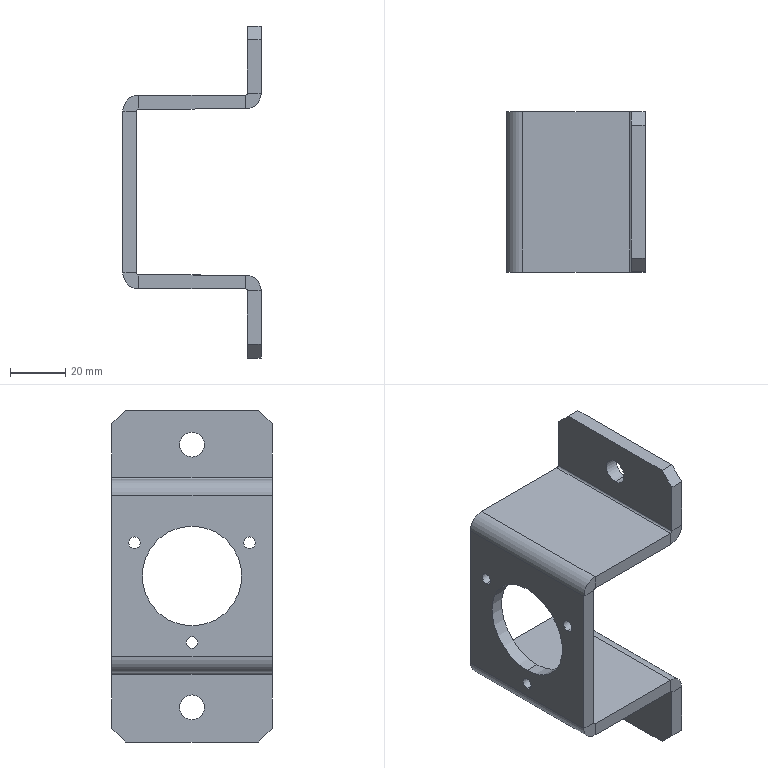Part | SolidWorks | features EdgeFlange 2, HoleWzd 2, Chamfer 1, CirPattern 1, FlatPattern 1, ICE 1, SMBaseFlange 1, SheetMetal 1 | 1 solid | 54 faces | box 50 x 58 x 120 mm | volume 53105 mm3 | plane 34 | cylinder 20 | commonest cylinder face diameters 4.2 x6 1.473 x4 9 x4 11.473 x4 36 x2
STEP:
#1=CARTESIAN_POINT('',(0.,20.785,14.1));
#2=VERTEX_POINT('',#1);
#3=CARTESIAN_POINT('',(0.,20.785,9.9));
#4=VERTEX_POINT('',#3);
#5=CARTESIAN_POINT('',(0.,20.785,12.));
#6=DIRECTION('',(1.,0.,0.));
#7=DIRECTION('',(0.,0.,-1.));
#8=AXIS2_PLACEMENT_3D('',#5,#6,#7);
#9=CIRCLE('',#8,2.1);
#10=EDGE_CURVE('',#2,#4,#9,.T.);
#11=ORIENTED_EDGE('',*,*,#10,.T.);
#12=CARTESIAN_POINT('',(-5.,20.785,9.9));
#13=VERTEX_POINT('',#12);
#14=CARTESIAN_POINT('',(-5.,20.785,9.9));
#15=DIRECTION('',(-1.,0.,0.));
#16=VECTOR('',#15,1000.);
#17=LINE('',#14,#16);
#18=EDGE_CURVE('',#4,#13,#17,.T.);
#19=ORIENTED_EDGE('',*,*,#18,.T.);
#20=CARTESIAN_POINT('',(-5.,20.785,14.1));
#21=VERTEX_POINT('',#20);
#22=CARTESIAN_POINT('',(-5.,20.785,12.));
#23=DIRECTION('',(-1.,0.,0.));
#24=DIRECTION('',(0.,0.,1.));
#25=AXIS2_PLACEMENT_3D('',#22,#23,#24);
#26=CIRCLE('',#25,2.1);
#27=EDGE_CURVE('',#13,#21,#26,.T.);
#28=ORIENTED_EDGE('',*,*,#27,.T.);
#29=CARTESIAN_POINT('',(-5.,20.785,14.1));
#30=DIRECTION('',(-1.,0.,0.));
#31=VECTOR('',#30,1000.);
#32=LINE('',#29,#31);
#33=EDGE_CURVE('',#2,#21,#32,.T.);
#34=ORIENTED_EDGE('',*,*,#33,.F.);
#35=EDGE_LOOP('',(#11,#19,#28,#34));
#36=FACE_OUTER_BOUND('',#35,.T.);
#37=CARTESIAN_POINT('',(-5.,20.785,12.));
#38=DIRECTION('',(-1.,0.,0.));
#39=DIRECTION('',(0.,0.,1.));
#40=AXIS2_PLACEMENT_3D('',#37,#38,#39);
#41=CYLINDRICAL_SURFACE('',#40,2.1);
#42=ADVANCED_FACE('',(#36),#41,.F.);
#43=CARTESIAN_POINT('',(0.,-20.785,14.1));
#44=VERTEX_POINT('',#43);
#45=CARTESIAN_POINT('',(0.,-20.785,9.9));
#46=VERTEX_POINT('',#45);
#47=CARTESIAN_POINT('',(0.,-20.785,12.));
#48=DIRECTION('',(1.,0.,0.));
#49=DIRECTION('',(0.,0.,-1.));
#50=AXIS2_PLACEMENT_3D('',#47,#48,#49);
#51=CIRCLE('',#50,2.1);
#52=EDGE_CURVE('',#44,#46,#51,.T.);
#53=ORIENTED_EDGE('',*,*,#52,.T.);
#54=CARTESIAN_POINT('',(-5.,-20.785,9.9));
#55=VERTEX_POINT('',#54);
#56=CARTESIAN_POINT('',(-5.,-20.785,9.9));
#57=DIRECTION('',(-1.,0.,0.));
#58=VECTOR('',#57,1000.);
#59=LINE('',#56,#58);
#60=EDGE_CURVE('',#46,#55,#59,.T.);
#61=ORIENTED_EDGE('',*,*,#60,.T.);
#62=CARTESIAN_POINT('',(-5.,-20.785,14.1));
#63=VERTEX_POINT('',#62);
#64=CARTESIAN_POINT('',(-5.,-20.785,12.));
#65=DIRECTION('',(-1.,0.,0.));
#66=DIRECTION('',(0.,0.,1.));
#67=AXIS2_PLACEMENT_3D('',#64,#65,#66);
#68=CIRCLE('',#67,2.1);
#69=EDGE_CURVE('',#55,#63,#68,.T.);
#70=ORIENTED_EDGE('',*,*,#69,.T.);
#71=CARTESIAN_POINT('',(-5.,-20.785,14.1));
#72=DIRECTION('',(-1.,0.,0.));
#73=VECTOR('',#72,1000.);
#74=LINE('',#71,#73);
#75=EDGE_CURVE('',#44,#63,#74,.T.);
#76=ORIENTED_EDGE('',*,*,#75,.F.);
#77=EDGE_LOOP('',(#53,#61,#70,#76));
#78=FACE_OUTER_BOUND('',#77,.T.);
#79=CARTESIAN_POINT('',(-5.,-20.785,12.));
#80=DIRECTION('',(-1.,0.,0.));
#81=DIRECTION('',(0.,0.,1.));
#82=AXIS2_PLACEMENT_3D('',#79,#80,#81);
#83=CYLINDRICAL_SURFACE('',#82,2.1);
#84=ADVANCED_FACE('',(#78),#83,.F.);
#85=CARTESIAN_POINT('',(0.,0.,-21.9));
#86=VERTEX_POINT('',#85);
#87=CARTESIAN_POINT('',(0.,0.,-26.1));
#88=VERTEX_POINT('',#87);
#89=CARTESIAN_POINT('',(0.,0.,-24.));
#90=DIRECTION('',(1.,0.,0.));
#91=DIRECTION('',(0.,0.,-1.));
#92=AXIS2_PLACEMENT_3D('',#89,#90,#91);
#93=CIRCLE('',#92,2.1);
#94=EDGE_CURVE('',#86,#88,#93,.T.);
#95=ORIENTED_EDGE('',*,*,#94,.T.);
#96=CARTESIAN_POINT('',(-5.,0.,-26.1));
#97=VERTEX_POINT('',#96);
#98=CARTESIAN_POINT('',(-5.,0.,-26.1));
#99=DIRECTION('',(-1.,0.,0.));
#100=VECTOR('',#99,1000.);
#101=LINE('',#98,#100);
#102=EDGE_CURVE('',#88,#97,#101,.T.);
#103=ORIENTED_EDGE('',*,*,#102,.T.);
#104=CARTESIAN_POINT('',(-5.,0.,-21.9));
#105=VERTEX_POINT('',#104);
#106=CARTESIAN_POINT('',(-5.,0.,-24.));
#107=DIRECTION('',(-1.,0.,0.));
#108=DIRECTION('',(0.,0.,1.));
#109=AXIS2_PLACEMENT_3D('',#106,#107,#108);
#110=CIRCLE('',#109,2.1);
#111=EDGE_CURVE('',#97,#105,#110,.T.);
#112=ORIENTED_EDGE('',*,*,#111,.T.);
#113=CARTESIAN_POINT('',(-5.,0.,-21.9));
#114=DIRECTION('',(-1.,0.,0.));
#115=VECTOR('',#114,1000.);
#116=LINE('',#113,#115);
#117=EDGE_CURVE('',#86,#105,#116,.T.);
#118=ORIENTED_EDGE('',*,*,#117,.F.);
#119=EDGE_LOOP('',(#95,#103,#112,#118));
#120=FACE_OUTER_BOUND('',#119,.T.);
#121=CARTESIAN_POINT('',(-5.,0.,-24.));
#122=DIRECTION('',(-1.,0.,0.));
#123=DIRECTION('',(0.,0.,1.));
#124=AXIS2_PLACEMENT_3D('',#121,#122,#123);
#125=CYLINDRICAL_SURFACE('',#124,2.1);
#126=ADVANCED_FACE('',(#120),#125,.F.);
#127=CARTESIAN_POINT('',(0.,0.,18.));
#128=VERTEX_POINT('',#127);
#129=CARTESIAN_POINT('',(0.,0.,-18.));
#130=VERTEX_POINT('',#129);
#131=CARTESIAN_POINT('',(0.,0.,0.));
#132=DIRECTION('',(1.,0.,0.));
#133=DIRECTION('',(0.,0.,-1.));
#134=AXIS2_PLACEMENT_3D('',#131,#132,#133);
#135=CIRCLE('',#134,18.);
#136=EDGE_CURVE('',#128,#130,#135,.T.);
#137=ORIENTED_EDGE('',*,*,#136,.T.);
#138=CARTESIAN_POINT('',(-5.,0.,-18.));
#139=VERTEX_POINT('',#138);
#140=CARTESIAN_POINT('',(45.,0.,-18.));
#141=DIRECTION('',(-1.,0.,0.));
#142=VECTOR('',#141,1000.);
#143=LINE('',#140,#142);
#144=EDGE_CURVE('',#130,#139,#143,.T.);
#145=ORIENTED_EDGE('',*,*,#144,.T.);
#146=CARTESIAN_POINT('',(-5.,0.,18.));
#147=VERTEX_POINT('',#146);
#148=CARTESIAN_POINT('',(-5.,0.,0.));
#149=DIRECTION('',(-1.,0.,0.));
#150=DIRECTION('',(0.,0.,1.));
#151=AXIS2_PLACEMENT_3D('',#148,#149,#150);
#152=CIRCLE('',#151,18.);
#153=EDGE_CURVE('',#139,#147,#152,.T.);
#154=ORIENTED_EDGE('',*,*,#153,.T.);
#155=CARTESIAN_POINT('',(45.,0.,18.));
#156=DIRECTION('',(-1.,0.,0.));
#157=VECTOR('',#156,1000.);
#158=LINE('',#155,#157);
#159=EDGE_CURVE('',#128,#147,#158,.T.);
#160=ORIENTED_EDGE('',*,*,#159,.F.);
#161=EDGE_LOOP('',(#137,#145,#154,#160));
#162=FACE_OUTER_BOUND('',#161,.T.);
#163=CARTESIAN_POINT('',(45.,0.,0.));
#164=DIRECTION('',(-1.,0.,0.));
#165=DIRECTION('',(0.,0.,1.));
#166=AXIS2_PLACEMENT_3D('',#163,#164,#165);
#167=CYLINDRICAL_SURFACE('',#166,18.);
#168=ADVANCED_FACE('',(#162),#167,.F.);
#169=CARTESIAN_POINT('',(45.,0.,-52.));
#170=VERTEX_POINT('',#169);
#171=CARTESIAN_POINT('',(45.,0.,-43.));
#172=VERTEX_POINT('',#171);
#173=CARTESIAN_POINT('',(45.,0.,-47.5));
#174=DIRECTION('',(-1.,0.,0.));
#175=DIRECTION('',(0.,0.,1.));
#176=AXIS2_PLACEMENT_3D('',#173,#174,#175);
#177=CIRCLE('',#176,4.5);
#178=EDGE_CURVE('',#170,#172,#177,.T.);
#179=ORIENTED_EDGE('',*,*,#178,.F.);
#180=CARTESIAN_POINT('',(40.,0.,-52.));
#181=VERTEX_POINT('',#180);
#182=CARTESIAN_POINT('',(40.,0.,-52.));
#183=DIRECTION('',(-1.,0.,0.));
#184=VECTOR('',#183,1000.);
#185=LINE('',#182,#184);
#186=EDGE_CURVE('',#170,#181,#185,.T.);
#187=ORIENTED_EDGE('',*,*,#186,.T.);
#188=CARTESIAN_POINT('',(40.,0.,-43.));
#189=VERTEX_POINT('',#188);
#190=CARTESIAN_POINT('',(40.,0.,-47.5));
#191=DIRECTION('',(-1.,0.,0.));
#192=DIRECTION('',(0.,0.,1.));
#193=AXIS2_PLACEMENT_3D('',#190,#191,#192);
#194=CIRCLE('',#193,4.5);
#195=EDGE_CURVE('',#181,#189,#194,.T.);
#196=ORIENTED_EDGE('',*,*,#195,.T.);
#197=CARTESIAN_POINT('',(40.,0.,-43.));
#198=DIRECTION('',(-1.,0.,0.));
#199=VECTOR('',#198,1000.);
#200=LINE('',#197,#199);
#201=EDGE_CURVE('',#172,#189,#200,.T.);
#202=ORIENTED_EDGE('',*,*,#201,.F.);
#203=EDGE_LOOP('',(#179,#187,#196,#202));
#204=FACE_OUTER_BOUND('',#203,.T.);
#205=CARTESIAN_POINT('',(40.,0.,-47.5));
#206=DIRECTION('',(-1.,0.,0.));
#207=DIRECTION('',(0.,0.,1.));
#208=AXIS2_PLACEMENT_3D('',#205,#206,#207);
#209=CYLINDRICAL_SURFACE('',#208,4.5);
#210=ADVANCED_FACE('',(#204),#209,.F.);
#211=CARTESIAN_POINT('',(45.,0.,43.));
#212=VERTEX_POINT('',#211);
#213=CARTESIAN_POINT('',(45.,0.,52.));
#214=VERTEX_POINT('',#213);
#215=CARTESIAN_POINT('',(45.,0.,47.5));
#216=DIRECTION('',(-1.,0.,0.));
#217=DIRECTION('',(0.,0.,1.));
#218=AXIS2_PLACEMENT_3D('',#215,#216,#217);
#219=CIRCLE('',#218,4.5);
#220=EDGE_CURVE('',#212,#214,#219,.T.);
#221=ORIENTED_EDGE('',*,*,#220,.F.);
#222=CARTESIAN_POINT('',(40.,0.,43.));
#223=VERTEX_POINT('',#222);
#224=CARTESIAN_POINT('',(40.,0.,43.));
#225=DIRECTION('',(-1.,0.,0.));
#226=VECTOR('',#225,1000.);
#227=LINE('',#224,#226);
#228=EDGE_CURVE('',#212,#223,#227,.T.);
#229=ORIENTED_EDGE('',*,*,#228,.T.);
#230=CARTESIAN_POINT('',(40.,0.,52.));
#231=VERTEX_POINT('',#230);
#232=CARTESIAN_POINT('',(40.,0.,47.5));
#233=DIRECTION('',(-1.,0.,0.));
#234=DIRECTION('',(0.,0.,1.));
#235=AXIS2_PLACEMENT_3D('',#232,#233,#234);
#236=CIRCLE('',#235,4.5);
#237=EDGE_CURVE('',#223,#231,#236,.T.);
#238=ORIENTED_EDGE('',*,*,#237,.T.);
#239=CARTESIAN_POINT('',(40.,0.,52.));
#240=DIRECTION('',(-1.,0.,0.));
#241=VECTOR('',#240,1000.);
#242=LINE('',#239,#241);
#243=EDGE_CURVE('',#214,#231,#242,.T.);
#244=ORIENTED_EDGE('',*,*,#243,.F.);
#245=EDGE_LOOP('',(#221,#229,#238,#244));
#246=FACE_OUTER_BOUND('',#245,.T.);
#247=CARTESIAN_POINT('',(40.,0.,47.5));
#248=DIRECTION('',(-1.,0.,0.));
#249=DIRECTION('',(0.,0.,1.));
#250=AXIS2_PLACEMENT_3D('',#247,#248,#249);
#251=CYLINDRICAL_SURFACE('',#250,4.5);
#252=ADVANCED_FACE('',(#246),#251,.F.);
#253=CARTESIAN_POINT('',(39.263,-29.,-35.));
#254=VERTEX_POINT('',#253);
#255=CARTESIAN_POINT('',(39.263,-29.,-30.));
#256=VERTEX_POINT('',#255);
#257=CARTESIAN_POINT('',(39.263,-29.,-35.));
#258=DIRECTION('',(0.,0.,1.));
#259=VECTOR('',#258,1000.);
#260=LINE('',#257,#259);
#261=EDGE_CURVE('',#254,#256,#260,.T.);
#262=ORIENTED_EDGE('',*,*,#261,.T.);
#263=CARTESIAN_POINT('',(0.7366,-29.,-30.));
#264=VERTEX_POINT('',#263);
#265=CARTESIAN_POINT('',(0.,-29.,-30.));
#266=DIRECTION('',(-1.,0.,0.));
#267=VECTOR('',#266,1000.);
#268=LINE('',#265,#267);
#269=EDGE_CURVE('',#256,#264,#268,.T.);
#270=ORIENTED_EDGE('',*,*,#269,.T.);
#271=CARTESIAN_POINT('',(0.7366,-29.,-35.));
#272=VERTEX_POINT('',#271);
#273=CARTESIAN_POINT('',(0.7366,-29.,-35.));
#274=DIRECTION('',(0.,0.,-1.));
#275=VECTOR('',#274,1000.);
#276=LINE('',#273,#275);
#277=EDGE_CURVE('',#264,#272,#276,.T.);
#278=ORIENTED_EDGE('',*,*,#277,.T.);
#279=CARTESIAN_POINT('',(0.,-29.,-35.));
#280=DIRECTION('',(-1.,0.,0.));
#281=VECTOR('',#280,1000.);
#282=LINE('',#279,#281);
#283=EDGE_CURVE('',#254,#272,#282,.T.);
#284=ORIENTED_EDGE('',*,*,#283,.F.);
#285=EDGE_LOOP('',(#262,#270,#278,#284));
#286=FACE_OUTER_BOUND('',#285,.T.);
#287=CARTESIAN_POINT('',(0.,-29.,-35.));
#288=DIRECTION('',(0.,1.,0.));
#289=DIRECTION('',(-1.,0.,0.));
#290=AXIS2_PLACEMENT_3D('',#287,#288,#289);
#291=PLANE('',#290);
#292=ADVANCED_FACE('',(#286),#291,.F.);
#293=CARTESIAN_POINT('',(39.263,29.,-35.));
#294=VERTEX_POINT('',#293);
#295=CARTESIAN_POINT('',(39.263,29.,-30.));
#296=VERTEX_POINT('',#295);
#297=CARTESIAN_POINT('',(39.263,29.,-35.));
#298=DIRECTION('',(0.,0.,1.));
#299=VECTOR('',#298,1000.);
#300=LINE('',#297,#299);
#301=EDGE_CURVE('',#294,#296,#300,.T.);
#302=ORIENTED_EDGE('',*,*,#301,.F.);
#303=CARTESIAN_POINT('',(0.7366,29.,-35.));
#304=VERTEX_POINT('',#303);
#305=CARTESIAN_POINT('',(0.,29.,-35.));
#306=DIRECTION('',(1.,0.,0.));
#307=VECTOR('',#306,1000.);
#308=LINE('',#305,#307);
#309=EDGE_CURVE('',#304,#294,#308,.T.);
#310=ORIENTED_EDGE('',*,*,#309,.F.);
#311=CARTESIAN_POINT('',(0.7366,29.,-30.));
#312=VERTEX_POINT('',#311);
#313=CARTESIAN_POINT('',(0.7366,29.,-30.));
#314=DIRECTION('',(0.,0.,-1.));
#315=VECTOR('',#314,1000.);
#316=LINE('',#313,#315);
#317=EDGE_CURVE('',#312,#304,#316,.T.);
#318=ORIENTED_EDGE('',*,*,#317,.F.);
#319=CARTESIAN_POINT('',(45.,29.,-30.));
#320=DIRECTION('',(1.,0.,0.));
#321=VECTOR('',#320,1000.);
#322=LINE('',#319,#321);
#323=EDGE_CURVE('',#312,#296,#322,.T.);
#324=ORIENTED_EDGE('',*,*,#323,.T.);
#325=EDGE_LOOP('',(#302,#310,#318,#324));
#326=FACE_OUTER_BOUND('',#325,.T.);
#327=CARTESIAN_POINT('',(45.,29.,-35.));
#328=DIRECTION('',(0.,-1.,0.));
#329=DIRECTION('',(1.,0.,0.));
#330=AXIS2_PLACEMENT_3D('',#327,#328,#329);
#331=PLANE('',#330);
#332=ADVANCED_FACE('',(#326),#331,.F.);
#333=CARTESIAN_POINT('',(39.263,-29.,-35.));
#334=DIRECTION('',(0.,1.,0.));
#335=VECTOR('',#334,1000.);
#336=LINE('',#333,#335);
#337=EDGE_CURVE('',#254,#294,#336,.T.);
#338=ORIENTED_EDGE('',*,*,#337,.F.);
#339=ORIENTED_EDGE('',*,*,#283,.T.);
#340=CARTESIAN_POINT('',(0.7366,-29.,-35.));
#341=DIRECTION('',(0.,-1.,0.));
#342=VECTOR('',#341,1000.);
#343=LINE('',#340,#342);
#344=EDGE_CURVE('',#304,#272,#343,.T.);
#345=ORIENTED_EDGE('',*,*,#344,.F.);
#346=ORIENTED_EDGE('',*,*,#309,.T.);
#347=EDGE_LOOP('',(#338,#339,#345,#346));
#348=FACE_OUTER_BOUND('',#347,.T.);
#349=CARTESIAN_POINT('',(0.,0.,-35.));
#350=DIRECTION('',(0.,0.,1.));
#351=DIRECTION('',(1.,0.,0.));
#352=AXIS2_PLACEMENT_3D('',#349,#350,#351);
#353=PLANE('',#352);
#354=ADVANCED_FACE('',(#348),#353,.F.);
#355=ORIENTED_EDGE('',*,*,#269,.F.);
#356=CARTESIAN_POINT('',(39.263,-29.,-30.));
#357=DIRECTION('',(0.,1.,0.));
#358=VECTOR('',#357,1000.);
#359=LINE('',#356,#358);
#360=EDGE_CURVE('',#256,#296,#359,.T.);
#361=ORIENTED_EDGE('',*,*,#360,.T.);
#362=ORIENTED_EDGE('',*,*,#323,.F.);
#363=CARTESIAN_POINT('',(0.7366,-29.,-30.));
#364=DIRECTION('',(0.,1.,0.));
#365=VECTOR('',#364,1000.);
#366=LINE('',#363,#365);
#367=EDGE_CURVE('',#264,#312,#366,.T.);
#368=ORIENTED_EDGE('',*,*,#367,.F.);
#369=EDGE_LOOP('',(#355,#361,#362,#368));
#370=FACE_OUTER_BOUND('',#369,.T.);
#371=CARTESIAN_POINT('',(0.,0.,-30.));
#372=DIRECTION('',(0.,0.,1.));
#373=DIRECTION('',(1.,0.,0.));
#374=AXIS2_PLACEMENT_3D('',#371,#372,#373);
#375=PLANE('',#374);
#376=ADVANCED_FACE('',(#370),#375,.T.);
#377=CARTESIAN_POINT('',(39.263,29.,35.));
#378=VERTEX_POINT('',#377);
#379=CARTESIAN_POINT('',(39.263,29.,30.));
#380=VERTEX_POINT('',#379);
#381=CARTESIAN_POINT('',(39.263,29.,35.));
#382=DIRECTION('',(0.,0.,-1.));
#383=VECTOR('',#382,1000.);
#384=LINE('',#381,#383);
#385=EDGE_CURVE('',#378,#380,#384,.T.);
#386=ORIENTED_EDGE('',*,*,#385,.T.);
#387=CARTESIAN_POINT('',(0.7366,29.,30.));
#388=VERTEX_POINT('',#387);
#389=CARTESIAN_POINT('',(0.,29.,30.));
#390=DIRECTION('',(-1.,0.,0.));
#391=VECTOR('',#390,1000.);
#392=LINE('',#389,#391);
#393=EDGE_CURVE('',#380,#388,#392,.T.);
#394=ORIENTED_EDGE('',*,*,#393,.T.);
#395=CARTESIAN_POINT('',(0.7366,29.,35.));
#396=VERTEX_POINT('',#395);
#397=CARTESIAN_POINT('',(0.7366,29.,35.));
#398=DIRECTION('',(0.,0.,1.));
#399=VECTOR('',#398,1000.);
#400=LINE('',#397,#399);
#401=EDGE_CURVE('',#388,#396,#400,.T.);
#402=ORIENTED_EDGE('',*,*,#401,.T.);
#403=CARTESIAN_POINT('',(0.,29.,35.));
#404=DIRECTION('',(-1.,0.,0.));
#405=VECTOR('',#404,1000.);
#406=LINE('',#403,#405);
#407=EDGE_CURVE('',#378,#396,#406,.T.);
#408=ORIENTED_EDGE('',*,*,#407,.F.);
#409=EDGE_LOOP('',(#386,#394,#402,#408));
#410=FACE_OUTER_BOUND('',#409,.T.);
#411=CARTESIAN_POINT('',(0.,29.,35.));
#412=DIRECTION('',(0.,-1.,0.));
#413=DIRECTION('',(1.,0.,0.));
#414=AXIS2_PLACEMENT_3D('',#411,#412,#413);
#415=PLANE('',#414);
#416=ADVANCED_FACE('',(#410),#415,.F.);
#417=CARTESIAN_POINT('',(39.263,-29.,35.));
#418=VERTEX_POINT('',#417);
#419=CARTESIAN_POINT('',(39.263,-29.,30.));
#420=VERTEX_POINT('',#419);
#421=CARTESIAN_POINT('',(39.263,-29.,35.));
#422=DIRECTION('',(0.,0.,-1.));
#423=VECTOR('',#422,1000.);
#424=LINE('',#421,#423);
#425=EDGE_CURVE('',#418,#420,#424,.T.);
#426=ORIENTED_EDGE('',*,*,#425,.F.);
#427=CARTESIAN_POINT('',(0.7366,-29.,35.));
#428=VERTEX_POINT('',#427);
#429=CARTESIAN_POINT('',(0.,-29.,35.));
#430=DIRECTION('',(1.,0.,0.));
#431=VECTOR('',#430,1000.);
#432=LINE('',#429,#431);
#433=EDGE_CURVE('',#428,#418,#432,.T.);
#434=ORIENTED_EDGE('',*,*,#433,.F.);
#435=CARTESIAN_POINT('',(0.7366,-29.,30.));
#436=VERTEX_POINT('',#435);
#437=CARTESIAN_POINT('',(0.7366,-29.,30.));
#438=DIRECTION('',(0.,0.,1.));
#439=VECTOR('',#438,1000.);
#440=LINE('',#437,#439);
#441=EDGE_CURVE('',#436,#428,#440,.T.);
#442=ORIENTED_EDGE('',*,*,#441,.F.);
#443=CARTESIAN_POINT('',(45.,-29.,30.));
#444=DIRECTION('',(1.,0.,0.));
#445=VECTOR('',#444,1000.);
#446=LINE('',#443,#445);
#447=EDGE_CURVE('',#436,#420,#446,.T.);
#448=ORIENTED_EDGE('',*,*,#447,.T.);
#449=EDGE_LOOP('',(#426,#434,#442,#448));
#450=FACE_OUTER_BOUND('',#449,.T.);
#451=CARTESIAN_POINT('',(45.,-29.,35.));
#452=DIRECTION('',(0.,1.,0.));
#453=DIRECTION('',(-1.,0.,0.));
#454=AXIS2_PLACEMENT_3D('',#451,#452,#453);
#455=PLANE('',#454);
#456=ADVANCED_FACE('',(#450),#455,.F.);
#457=CARTESIAN_POINT('',(39.263,29.,35.));
#458=DIRECTION('',(0.,-1.,0.));
#459=VECTOR('',#458,1000.);
#460=LINE('',#457,#459);
#461=EDGE_CURVE('',#378,#418,#460,.T.);
#462=ORIENTED_EDGE('',*,*,#461,.F.);
#463=ORIENTED_EDGE('',*,*,#407,.T.);
#464=CARTESIAN_POINT('',(0.7366,29.,35.));
#465=DIRECTION('',(0.,1.,0.));
#466=VECTOR('',#465,1000.);
#467=LINE('',#464,#466);
#468=EDGE_CURVE('',#428,#396,#467,.T.);
#469=ORIENTED_EDGE('',*,*,#468,.F.);
#470=ORIENTED_EDGE('',*,*,#433,.T.);
#471=EDGE_LOOP('',(#462,#463,#469,#470));
#472=FACE_OUTER_BOUND('',#471,.T.);
#473=CARTESIAN_POINT('',(0.,0.,35.));
#474=DIRECTION('',(0.,0.,-1.));
#475=DIRECTION('',(-1.,0.,0.));
#476=AXIS2_PLACEMENT_3D('',#473,#474,#475);
#477=PLANE('',#476);
#478=ADVANCED_FACE('',(#472),#477,.F.);
#479=ORIENTED_EDGE('',*,*,#393,.F.);
#480=CARTESIAN_POINT('',(39.263,29.,30.));
#481=DIRECTION('',(0.,-1.,0.));
#482=VECTOR('',#481,1000.);
#483=LINE('',#480,#482);
#484=EDGE_CURVE('',#380,#420,#483,.T.);
#485=ORIENTED_EDGE('',*,*,#484,.T.);
#486=ORIENTED_EDGE('',*,*,#447,.F.);
#487=CARTESIAN_POINT('',(0.7366,29.,30.));
#488=DIRECTION('',(0.,-1.,0.));
#489=VECTOR('',#488,1000.);
#490=LINE('',#487,#489);
#491=EDGE_CURVE('',#388,#436,#490,.T.);
#492=ORIENTED_EDGE('',*,*,#491,.F.);
#493=EDGE_LOOP('',(#479,#485,#486,#492));
#494=FACE_OUTER_BOUND('',#493,.T.);
#495=CARTESIAN_POINT('',(0.,0.,30.));
#496=DIRECTION('',(0.,0.,-1.));
#497=DIRECTION('',(-1.,0.,0.));
#498=AXIS2_PLACEMENT_3D('',#495,#496,#497);
#499=PLANE('',#498);
#500=ADVANCED_FACE('',(#494),#499,.T.);
#501=CARTESIAN_POINT('',(-5.,20.785,12.));
#502=DIRECTION('',(-1.,0.,0.));
#503=DIRECTION('',(0.,0.,1.));
#504=AXIS2_PLACEMENT_3D('',#501,#502,#503);
#505=CIRCLE('',#504,2.1);
#506=EDGE_CURVE('',#21,#13,#505,.T.);
#507=ORIENTED_EDGE('',*,*,#506,.F.);
#508=ORIENTED_EDGE('',*,*,#27,.F.);
#509=EDGE_LOOP('',(#507,#508));
#510=FACE_BOUND('',#509,.T.);
#511=CARTESIAN_POINT('',(-5.,-20.785,12.));
#512=DIRECTION('',(-1.,0.,0.));
#513=DIRECTION('',(0.,0.,1.));
#514=AXIS2_PLACEMENT_3D('',#511,#512,#513);
#515=CIRCLE('',#514,2.1);
#516=EDGE_CURVE('',#63,#55,#515,.T.);
#517=ORIENTED_EDGE('',*,*,#516,.F.);
#518=ORIENTED_EDGE('',*,*,#69,.F.);
#519=EDGE_LOOP('',(#517,#518));
#520=FACE_BOUND('',#519,.T.);
#521=CARTESIAN_POINT('',(-5.,0.,-24.));
#522=DIRECTION('',(-1.,0.,0.));
#523=DIRECTION('',(0.,0.,1.));
#524=AXIS2_PLACEMENT_3D('',#521,#522,#523);
#525=CIRCLE('',#524,2.1);
#526=EDGE_CURVE('',#105,#97,#525,.T.);
#527=ORIENTED_EDGE('',*,*,#526,.F.);
#528=ORIENTED_EDGE('',*,*,#111,.F.);
#529=EDGE_LOOP('',(#527,#528));
#530=FACE_BOUND('',#529,.T.);
#531=CARTESIAN_POINT('',(-5.,0.,0.));
#532=DIRECTION('',(-1.,0.,0.));
#533=DIRECTION('',(0.,0.,1.));
#534=AXIS2_PLACEMENT_3D('',#531,#532,#533);
#535=CIRCLE('',#534,18.);
#536=EDGE_CURVE('',#147,#139,#535,.T.);
#537=ORIENTED_EDGE('',*,*,#536,.F.);
#538=ORIENTED_EDGE('',*,*,#153,.F.);
#539=EDGE_LOOP('',(#537,#538));
#540=FACE_BOUND('',#539,.T.);
#541=CARTESIAN_POINT('',(-5.,29.,-29.263));
#542=VERTEX_POINT('',#541);
#543=CARTESIAN_POINT('',(-5.,-29.,-29.263));
#544=VERTEX_POINT('',#543);
#545=CARTESIAN_POINT('',(-5.,29.,-29.263));
#546=DIRECTION('',(0.,-1.,0.));
#547=VECTOR('',#546,1000.);
#548=LINE('',#545,#547);
#549=EDGE_CURVE('',#542,#544,#548,.T.);
#550=ORIENTED_EDGE('',*,*,#549,.T.);
#551=CARTESIAN_POINT('',(-5.,-29.,29.263));
#552=VERTEX_POINT('',#551);
#553=CARTESIAN_POINT('',(-5.,-29.,35.));
#554=DIRECTION('',(0.,0.,-1.));
#555=VECTOR('',#554,1000.);
#556=LINE('',#553,#555);
#557=EDGE_CURVE('',#552,#544,#556,.T.);
#558=ORIENTED_EDGE('',*,*,#557,.F.);
#559=CARTESIAN_POINT('',(-5.,29.,29.263));
#560=VERTEX_POINT('',#559);
#561=CARTESIAN_POINT('',(-5.,-29.,29.263));
#562=DIRECTION('',(0.,1.,0.));
#563=VECTOR('',#562,1000.);
#564=LINE('',#561,#563);
#565=EDGE_CURVE('',#552,#560,#564,.T.);
#566=ORIENTED_EDGE('',*,*,#565,.T.);
#567=CARTESIAN_POINT('',(-5.,29.,35.));
#568=DIRECTION('',(0.,0.,1.));
#569=VECTOR('',#568,1000.);
#570=LINE('',#567,#569);
#571=EDGE_CURVE('',#542,#560,#570,.T.);
#572=ORIENTED_EDGE('',*,*,#571,.F.);
#573=EDGE_LOOP('',(#550,#558,#566,#572));
#574=FACE_OUTER_BOUND('',#573,.T.);
#575=CARTESIAN_POINT('',(-5.,0.,0.));
#576=DIRECTION('',(1.,0.,0.));
#577=DIRECTION('',(0.,0.,-1.));
#578=AXIS2_PLACEMENT_3D('',#575,#576,#577);
#579=PLANE('',#578);
#580=ADVANCED_FACE('',(#510,#520,#530,#540,#574),#579,.F.);
#581=ORIENTED_EDGE('',*,*,#10,.F.);
#582=CARTESIAN_POINT('',(0.,20.785,12.));
#583=DIRECTION('',(1.,0.,0.));
#584=DIRECTION('',(0.,0.,-1.));
#585=AXIS2_PLACEMENT_3D('',#582,#583,#584);
#586=CIRCLE('',#585,2.1);
#587=EDGE_CURVE('',#4,#2,#586,.T.);
#588=ORIENTED_EDGE('',*,*,#587,.F.);
#589=EDGE_LOOP('',(#581,#588));
#590=FACE_BOUND('',#589,.T.);
#591=ORIENTED_EDGE('',*,*,#52,.F.);
#592=CARTESIAN_POINT('',(0.,-20.785,12.));
#593=DIRECTION('',(1.,0.,0.));
#594=DIRECTION('',(0.,0.,-1.));
#595=AXIS2_PLACEMENT_3D('',#592,#593,#594);
#596=CIRCLE('',#595,2.1);
#597=EDGE_CURVE('',#46,#44,#596,.T.);
#598=ORIENTED_EDGE('',*,*,#597,.F.);
#599=EDGE_LOOP('',(#591,#598));
#600=FACE_BOUND('',#599,.T.);
#601=ORIENTED_EDGE('',*,*,#94,.F.);
#602=CARTESIAN_POINT('',(0.,0.,-24.));
#603=DIRECTION('',(1.,0.,0.));
#604=DIRECTION('',(0.,0.,-1.));
#605=AXIS2_PLACEMENT_3D('',#602,#603,#604);
#606=CIRCLE('',#605,2.1);
#607=EDGE_CURVE('',#88,#86,#606,.T.);
#608=ORIENTED_EDGE('',*,*,#607,.F.);
#609=EDGE_LOOP('',(#601,#608));
#610=FACE_BOUND('',#609,.T.);
#611=ORIENTED_EDGE('',*,*,#136,.F.);
#612=CARTESIAN_POINT('',(0.,0.,0.));
#613=DIRECTION('',(1.,0.,0.));
#614=DIRECTION('',(0.,0.,-1.));
#615=AXIS2_PLACEMENT_3D('',#612,#613,#614);
#616=CIRCLE('',#615,18.);
#617=EDGE_CURVE('',#130,#128,#616,.T.);
#618=ORIENTED_EDGE('',*,*,#617,.F.);
#619=EDGE_LOOP('',(#611,#618));
#620=FACE_BOUND('',#619,.T.);
#621=CARTESIAN_POINT('',(0.,-29.,29.263));
#622=VERTEX_POINT('',#621);
#623=CARTESIAN_POINT('',(0.,-29.,-29.263));
#624=VERTEX_POINT('',#623);
#625=CARTESIAN_POINT('',(0.,-29.,35.));
#626=DIRECTION('',(0.,0.,-1.));
#627=VECTOR('',#626,1000.);
#628=LINE('',#625,#627);
#629=EDGE_CURVE('',#622,#624,#628,.T.);
#630=ORIENTED_EDGE('',*,*,#629,.T.);
#631=CARTESIAN_POINT('',(0.,29.,-29.263));
#632=VERTEX_POINT('',#631);
#633=CARTESIAN_POINT('',(0.,29.,-29.263));
#634=DIRECTION('',(0.,-1.,0.));
#635=VECTOR('',#634,1000.);
#636=LINE('',#633,#635);
#637=EDGE_CURVE('',#632,#624,#636,.T.);
#638=ORIENTED_EDGE('',*,*,#637,.F.);
#639=CARTESIAN_POINT('',(0.,29.,29.263));
#640=VERTEX_POINT('',#639);
#641=CARTESIAN_POINT('',(0.,29.,35.));
#642=DIRECTION('',(0.,0.,1.));
#643=VECTOR('',#642,1000.);
#644=LINE('',#641,#643);
#645=EDGE_CURVE('',#632,#640,#644,.T.);
#646=ORIENTED_EDGE('',*,*,#645,.T.);
#647=CARTESIAN_POINT('',(0.,-29.,29.263));
#648=DIRECTION('',(0.,1.,0.));
#649=VECTOR('',#648,1000.);
#650=LINE('',#647,#649);
#651=EDGE_CURVE('',#622,#640,#650,.T.);
#652=ORIENTED_EDGE('',*,*,#651,.F.);
#653=EDGE_LOOP('',(#630,#638,#646,#652));
#654=FACE_OUTER_BOUND('',#653,.T.);
#655=CARTESIAN_POINT('',(0.,0.,0.));
#656=DIRECTION('',(1.,0.,0.));
#657=DIRECTION('',(0.,0.,-1.));
#658=AXIS2_PLACEMENT_3D('',#655,#656,#657);
#659=PLANE('',#658);
#660=ADVANCED_FACE('',(#590,#600,#610,#620,#654),#659,.T.);
#661=ORIENTED_EDGE('',*,*,#645,.F.);
#662=CARTESIAN_POINT('',(0.,29.,-29.263));
#663=DIRECTION('',(-1.,0.,0.));
#664=VECTOR('',#663,1000.);
#665=LINE('',#662,#664);
#666=EDGE_CURVE('',#632,#542,#665,.T.);
#667=ORIENTED_EDGE('',*,*,#666,.T.);
#668=ORIENTED_EDGE('',*,*,#571,.T.);
#669=CARTESIAN_POINT('',(0.,29.,29.263));
#670=DIRECTION('',(-1.,0.,0.));
#671=VECTOR('',#670,1000.);
#672=LINE('',#669,#671);
#673=EDGE_CURVE('',#640,#560,#672,.T.);
#674=ORIENTED_EDGE('',*,*,#673,.F.);
#675=EDGE_LOOP('',(#661,#667,#668,#674));
#676=FACE_OUTER_BOUND('',#675,.T.);
#677=CARTESIAN_POINT('',(-5.,29.,35.));
#678=DIRECTION('',(0.,1.,0.));
#679=DIRECTION('',(0.,0.,1.));
#680=AXIS2_PLACEMENT_3D('',#677,#678,#679);
#681=PLANE('',#680);
#682=ADVANCED_FACE('',(#676),#681,.T.);
#683=CARTESIAN_POINT('',(0.,-29.,-29.263));
#684=DIRECTION('',(-1.,0.,0.));
#685=VECTOR('',#684,1000.);
#686=LINE('',#683,#685);
#687=EDGE_CURVE('',#624,#544,#686,.T.);
#688=ORIENTED_EDGE('',*,*,#687,.F.);
#689=ORIENTED_EDGE('',*,*,#629,.F.);
#690=CARTESIAN_POINT('',(0.,-29.,29.263));
#691=DIRECTION('',(-1.,0.,0.));
#692=VECTOR('',#691,1000.);
#693=LINE('',#690,#692);
#694=EDGE_CURVE('',#622,#552,#693,.T.);
#695=ORIENTED_EDGE('',*,*,#694,.T.);
#696=ORIENTED_EDGE('',*,*,#557,.T.);
#697=EDGE_LOOP('',(#688,#689,#695,#696));
#698=FACE_OUTER_BOUND('',#697,.T.);
#699=CARTESIAN_POINT('',(-5.,-29.,35.));
#700=DIRECTION('',(0.,-1.,0.));
#701=DIRECTION('',(0.,0.,-1.));
#702=AXIS2_PLACEMENT_3D('',#699,#700,#701);
#703=PLANE('',#702);
#704=ADVANCED_FACE('',(#698),#703,.T.);
#705=ORIENTED_EDGE('',*,*,#401,.F.);
#706=CARTESIAN_POINT('',(0.7366,29.,29.263));
#707=DIRECTION('',(0.,1.,0.));
#708=DIRECTION('',(1.,0.,0.));
#709=AXIS2_PLACEMENT_3D('',#706,#707,#708);
#710=CIRCLE('',#709,0.7366);
#711=EDGE_CURVE('',#640,#388,#710,.T.);
#712=ORIENTED_EDGE('',*,*,#711,.F.);
#713=ORIENTED_EDGE('',*,*,#673,.T.);
#714=CARTESIAN_POINT('',(0.7366,29.,29.263));
#715=DIRECTION('',(0.,1.,0.));
#716=DIRECTION('',(1.,0.,0.));
#717=AXIS2_PLACEMENT_3D('',#714,#715,#716);
#718=CIRCLE('',#717,5.737);
#719=EDGE_CURVE('',#560,#396,#718,.T.);
#720=ORIENTED_EDGE('',*,*,#719,.T.);
#721=EDGE_LOOP('',(#705,#712,#713,#720));
#722=FACE_OUTER_BOUND('',#721,.T.);
#723=CARTESIAN_POINT('',(0.7366,29.,29.263));
#724=DIRECTION('',(0.,1.,0.));
#725=DIRECTION('',(-1.,0.,0.));
#726=AXIS2_PLACEMENT_3D('',#723,#724,#725);
#727=PLANE('',#726);
#728=ADVANCED_FACE('',(#722),#727,.T.);
#729=CARTESIAN_POINT('',(0.7366,-29.,29.263));
#730=DIRECTION('',(0.,-1.,0.));
#731=DIRECTION('',(1.,0.,0.));
#732=AXIS2_PLACEMENT_3D('',#729,#730,#731);
#733=CIRCLE('',#732,0.7366);
#734=EDGE_CURVE('',#436,#622,#733,.T.);
#735=ORIENTED_EDGE('',*,*,#734,.F.);
#736=ORIENTED_EDGE('',*,*,#441,.T.);
#737=CARTESIAN_POINT('',(0.7366,-29.,29.263));
#738=DIRECTION('',(0.,-1.,0.));
#739=DIRECTION('',(1.,0.,0.));
#740=AXIS2_PLACEMENT_3D('',#737,#738,#739);
#741=CIRCLE('',#740,5.737);
#742=EDGE_CURVE('',#428,#552,#741,.T.);
#743=ORIENTED_EDGE('',*,*,#742,.T.);
#744=ORIENTED_EDGE('',*,*,#694,.F.);
#745=EDGE_LOOP('',(#735,#736,#743,#744));
#746=FACE_OUTER_BOUND('',#745,.T.);
#747=CARTESIAN_POINT('',(0.7366,-29.,29.263));
#748=DIRECTION('',(0.,1.,0.));
#749=DIRECTION('',(-1.,0.,0.));
#750=AXIS2_PLACEMENT_3D('',#747,#748,#749);
#751=PLANE('',#750);
#752=ADVANCED_FACE('',(#746),#751,.F.);
#753=ORIENTED_EDGE('',*,*,#565,.F.);
#754=ORIENTED_EDGE('',*,*,#742,.F.);
#755=ORIENTED_EDGE('',*,*,#468,.T.);
#756=ORIENTED_EDGE('',*,*,#719,.F.);
#757=EDGE_LOOP('',(#753,#754,#755,#756));
#758=FACE_OUTER_BOUND('',#757,.T.);
#759=CARTESIAN_POINT('',(0.7366,-29.,29.263));
#760=DIRECTION('',(0.,-1.,0.));
#761=DIRECTION('',(0.,0.,1.));
#762=AXIS2_PLACEMENT_3D('',#759,#760,#761);
#763=CYLINDRICAL_SURFACE('',#762,5.737);
#764=ADVANCED_FACE('',(#758),#763,.T.);
#765=ORIENTED_EDGE('',*,*,#651,.T.);
#766=ORIENTED_EDGE('',*,*,#711,.T.);
#767=ORIENTED_EDGE('',*,*,#491,.T.);
#768=ORIENTED_EDGE('',*,*,#734,.T.);
#769=EDGE_LOOP('',(#765,#766,#767,#768));
#770=FACE_OUTER_BOUND('',#769,.T.);
#771=CARTESIAN_POINT('',(0.7366,-29.,29.263));
#772=DIRECTION('',(0.,-1.,0.));
#773=DIRECTION('',(0.,0.,1.));
#774=AXIS2_PLACEMENT_3D('',#771,#772,#773);
#775=CYLINDRICAL_SURFACE('',#774,0.7366);
#776=ADVANCED_FACE('',(#770),#775,.F.);
#777=ORIENTED_EDGE('',*,*,#277,.F.);
#778=CARTESIAN_POINT('',(0.7366,-29.,-29.263));
#779=DIRECTION('',(0.,-1.,0.));
#780=DIRECTION('',(-1.,0.,0.));
#781=AXIS2_PLACEMENT_3D('',#778,#779,#780);
#782=CIRCLE('',#781,0.7366);
#783=EDGE_CURVE('',#624,#264,#782,.T.);
#784=ORIENTED_EDGE('',*,*,#783,.F.);
#785=ORIENTED_EDGE('',*,*,#687,.T.);
#786=CARTESIAN_POINT('',(0.7366,-29.,-29.263));
#787=DIRECTION('',(0.,-1.,0.));
#788=DIRECTION('',(-1.,0.,0.));
#789=AXIS2_PLACEMENT_3D('',#786,#787,#788);
#790=CIRCLE('',#789,5.737);
#791=EDGE_CURVE('',#544,#272,#790,.T.);
#792=ORIENTED_EDGE('',*,*,#791,.T.);
#793=EDGE_LOOP('',(#777,#784,#785,#792));
#794=FACE_OUTER_BOUND('',#793,.T.);
#795=CARTESIAN_POINT('',(0.7366,-29.,-29.263));
#796=DIRECTION('',(0.,-1.,0.));
#797=DIRECTION('',(1.,0.,0.));
#798=AXIS2_PLACEMENT_3D('',#795,#796,#797);
#799=PLANE('',#798);
#800=ADVANCED_FACE('',(#794),#799,.T.);
#801=CARTESIAN_POINT('',(0.7366,29.,-29.263));
#802=DIRECTION('',(0.,1.,0.));
#803=DIRECTION('',(-1.,0.,0.));
#804=AXIS2_PLACEMENT_3D('',#801,#802,#803);
#805=CIRCLE('',#804,0.7366);
#806=EDGE_CURVE('',#312,#632,#805,.T.);
#807=ORIENTED_EDGE('',*,*,#806,.F.);
#808=ORIENTED_EDGE('',*,*,#317,.T.);
#809=CARTESIAN_POINT('',(0.7366,29.,-29.263));
#810=DIRECTION('',(0.,1.,0.));
#811=DIRECTION('',(-1.,0.,0.));
#812=AXIS2_PLACEMENT_3D('',#809,#810,#811);
#813=CIRCLE('',#812,5.737);
#814=EDGE_CURVE('',#304,#542,#813,.T.);
#815=ORIENTED_EDGE('',*,*,#814,.T.);
#816=ORIENTED_EDGE('',*,*,#666,.F.);
#817=EDGE_LOOP('',(#807,#808,#815,#816));
#818=FACE_OUTER_BOUND('',#817,.T.);
#819=CARTESIAN_POINT('',(0.7366,29.,-29.263));
#820=DIRECTION('',(0.,-1.,0.));
#821=DIRECTION('',(1.,0.,0.));
#822=AXIS2_PLACEMENT_3D('',#819,#820,#821);
#823=PLANE('',#822);
#824=ADVANCED_FACE('',(#818),#823,.F.);
#825=ORIENTED_EDGE('',*,*,#549,.F.);
#826=ORIENTED_EDGE('',*,*,#814,.F.);
#827=ORIENTED_EDGE('',*,*,#344,.T.);
#828=ORIENTED_EDGE('',*,*,#791,.F.);
#829=EDGE_LOOP('',(#825,#826,#827,#828));
#830=FACE_OUTER_BOUND('',#829,.T.);
#831=CARTESIAN_POINT('',(0.7366,29.,-29.263));
#832=DIRECTION('',(0.,1.,0.));
#833=DIRECTION('',(0.,0.,-1.));
#834=AXIS2_PLACEMENT_3D('',#831,#832,#833);
#835=CYLINDRICAL_SURFACE('',#834,5.737);
#836=ADVANCED_FACE('',(#830),#835,.T.);
#837=ORIENTED_EDGE('',*,*,#637,.T.);
#838=ORIENTED_EDGE('',*,*,#783,.T.);
#839=ORIENTED_EDGE('',*,*,#367,.T.);
#840=ORIENTED_EDGE('',*,*,#806,.T.);
#841=EDGE_LOOP('',(#837,#838,#839,#840));
#842=FACE_OUTER_BOUND('',#841,.T.);
#843=CARTESIAN_POINT('',(0.7366,29.,-29.263));
#844=DIRECTION('',(0.,1.,0.));
#845=DIRECTION('',(0.,0.,-1.));
#846=AXIS2_PLACEMENT_3D('',#843,#844,#845);
#847=CYLINDRICAL_SURFACE('',#846,0.7366);
#848=ADVANCED_FACE('',(#842),#847,.F.);
#849=CARTESIAN_POINT('',(40.,-29.,35.737));
#850=VERTEX_POINT('',#849);
#851=CARTESIAN_POINT('',(45.,-29.,35.737));
#852=VERTEX_POINT('',#851);
#853=CARTESIAN_POINT('',(45.,-29.,35.737));
#854=DIRECTION('',(1.,0.,0.));
#855=VECTOR('',#854,1000.);
#856=LINE('',#853,#855);
#857=EDGE_CURVE('',#850,#852,#856,.T.);
#858=ORIENTED_EDGE('',*,*,#857,.F.);
#859=CARTESIAN_POINT('',(39.263,-29.,35.737));
#860=DIRECTION('',(0.,-1.,0.));
#861=DIRECTION('',(0.,0.,1.));
#862=AXIS2_PLACEMENT_3D('',#859,#860,#861);
#863=CIRCLE('',#862,0.7366);
#864=EDGE_CURVE('',#418,#850,#863,.T.);
#865=ORIENTED_EDGE('',*,*,#864,.F.);
#866=ORIENTED_EDGE('',*,*,#425,.T.);
#867=CARTESIAN_POINT('',(39.263,-29.,35.737));
#868=DIRECTION('',(0.,-1.,0.));
#869=DIRECTION('',(0.,0.,1.));
#870=AXIS2_PLACEMENT_3D('',#867,#868,#869);
#871=CIRCLE('',#870,5.737);
#872=EDGE_CURVE('',#420,#852,#871,.T.);
#873=ORIENTED_EDGE('',*,*,#872,.T.);
#874=EDGE_LOOP('',(#858,#865,#866,#873));
#875=FACE_OUTER_BOUND('',#874,.T.);
#876=CARTESIAN_POINT('',(39.263,-29.,35.737));
#877=DIRECTION('',(0.,-1.,0.));
#878=DIRECTION('',(0.,0.,-1.));
#879=AXIS2_PLACEMENT_3D('',#876,#877,#878);
#880=PLANE('',#879);
#881=ADVANCED_FACE('',(#875),#880,.T.);
#882=CARTESIAN_POINT('',(40.,29.,35.737));
#883=VERTEX_POINT('',#882);
#884=CARTESIAN_POINT('',(39.263,29.,35.737));
#885=DIRECTION('',(0.,1.,0.));
#886=DIRECTION('',(0.,0.,1.));
#887=AXIS2_PLACEMENT_3D('',#884,#885,#886);
#888=CIRCLE('',#887,0.7366);
#889=EDGE_CURVE('',#883,#378,#888,.T.);
#890=ORIENTED_EDGE('',*,*,#889,.F.);
#891=CARTESIAN_POINT('',(45.,29.,35.737));
#892=VERTEX_POINT('',#891);
#893=CARTESIAN_POINT('',(40.,29.,35.737));
#894=DIRECTION('',(1.,0.,0.));
#895=VECTOR('',#894,1000.);
#896=LINE('',#893,#895);
#897=EDGE_CURVE('',#883,#892,#896,.T.);
#898=ORIENTED_EDGE('',*,*,#897,.T.);
#899=CARTESIAN_POINT('',(39.263,29.,35.737));
#900=DIRECTION('',(0.,1.,0.));
#901=DIRECTION('',(0.,0.,1.));
#902=AXIS2_PLACEMENT_3D('',#899,#900,#901);
#903=CIRCLE('',#902,5.737);
#904=EDGE_CURVE('',#892,#380,#903,.T.);
#905=ORIENTED_EDGE('',*,*,#904,.T.);
#906=ORIENTED_EDGE('',*,*,#385,.F.);
#907=EDGE_LOOP('',(#890,#898,#905,#906));
#908=FACE_OUTER_BOUND('',#907,.T.);
#909=CARTESIAN_POINT('',(39.263,29.,35.737));
#910=DIRECTION('',(0.,-1.,0.));
#911=DIRECTION('',(0.,0.,-1.));
#912=AXIS2_PLACEMENT_3D('',#909,#910,#911);
#913=PLANE('',#912);
#914=ADVANCED_FACE('',(#908),#913,.F.);
#915=ORIENTED_EDGE('',*,*,#484,.F.);
#916=ORIENTED_EDGE('',*,*,#904,.F.);
#917=CARTESIAN_POINT('',(45.,-29.,35.737));
#918=DIRECTION('',(0.,-1.,0.));
#919=VECTOR('',#918,1000.);
#920=LINE('',#917,#919);
#921=EDGE_CURVE('',#892,#852,#920,.T.);
#922=ORIENTED_EDGE('',*,*,#921,.T.);
#923=ORIENTED_EDGE('',*,*,#872,.F.);
#924=EDGE_LOOP('',(#915,#916,#922,#923));
#925=FACE_OUTER_BOUND('',#924,.T.);
#926=CARTESIAN_POINT('',(39.263,29.,35.737));
#927=DIRECTION('',(0.,1.,0.));
#928=DIRECTION('',(1.,0.,0.));
#929=AXIS2_PLACEMENT_3D('',#926,#927,#928);
#930=CYLINDRICAL_SURFACE('',#929,5.737);
#931=ADVANCED_FACE('',(#925),#930,.T.);
#932=ORIENTED_EDGE('',*,*,#461,.T.);
#933=ORIENTED_EDGE('',*,*,#864,.T.);
#934=CARTESIAN_POINT('',(40.,-29.,35.737));
#935=DIRECTION('',(0.,1.,0.));
#936=VECTOR('',#935,1000.);
#937=LINE('',#934,#936);
#938=EDGE_CURVE('',#850,#883,#937,.T.);
#939=ORIENTED_EDGE('',*,*,#938,.T.);
#940=ORIENTED_EDGE('',*,*,#889,.T.);
#941=EDGE_LOOP('',(#932,#933,#939,#940));
#942=FACE_OUTER_BOUND('',#941,.T.);
#943=CARTESIAN_POINT('',(39.263,29.,35.737));
#944=DIRECTION('',(0.,1.,0.));
#945=DIRECTION('',(1.,0.,0.));
#946=AXIS2_PLACEMENT_3D('',#943,#944,#945);
#947=CYLINDRICAL_SURFACE('',#946,0.7366);
#948=ADVANCED_FACE('',(#942),#947,.F.);
#949=CARTESIAN_POINT('',(40.,29.,55.));
#950=VERTEX_POINT('',#949);
#951=CARTESIAN_POINT('',(40.,29.,60.));
#952=DIRECTION('',(0.,0.,1.));
#953=VECTOR('',#952,1000.);
#954=LINE('',#951,#953);
#955=EDGE_CURVE('',#883,#950,#954,.T.);
#956=ORIENTED_EDGE('',*,*,#955,.T.);
#957=CARTESIAN_POINT('',(45.,29.,55.));
#958=VERTEX_POINT('',#957);
#959=CARTESIAN_POINT('',(45.,29.,55.));
#960=DIRECTION('',(1.,0.,0.));
#961=VECTOR('',#960,1000.);
#962=LINE('',#959,#961);
#963=EDGE_CURVE('',#950,#958,#962,.T.);
#964=ORIENTED_EDGE('',*,*,#963,.T.);
#965=CARTESIAN_POINT('',(45.,29.,0.));
#966=DIRECTION('',(0.,0.,1.));
#967=VECTOR('',#966,1000.);
#968=LINE('',#965,#967);
#969=EDGE_CURVE('',#892,#958,#968,.T.);
#970=ORIENTED_EDGE('',*,*,#969,.F.);
#971=ORIENTED_EDGE('',*,*,#897,.F.);
#972=EDGE_LOOP('',(#956,#964,#970,#971));
#973=FACE_OUTER_BOUND('',#972,.T.);
#974=CARTESIAN_POINT('',(45.,29.,60.));
#975=DIRECTION('',(0.,-1.,0.));
#976=DIRECTION('',(0.,0.,-1.));
#977=AXIS2_PLACEMENT_3D('',#974,#975,#976);
#978=PLANE('',#977);
#979=ADVANCED_FACE('',(#973),#978,.F.);
#980=CARTESIAN_POINT('',(45.,-29.,55.));
#981=VERTEX_POINT('',#980);
#982=CARTESIAN_POINT('',(45.,-29.,0.));
#983=DIRECTION('',(0.,0.,-1.));
#984=VECTOR('',#983,1000.);
#985=LINE('',#982,#984);
#986=EDGE_CURVE('',#981,#852,#985,.T.);
#987=ORIENTED_EDGE('',*,*,#986,.F.);
#988=CARTESIAN_POINT('',(40.,-29.,55.));
#989=VERTEX_POINT('',#988);
#990=CARTESIAN_POINT('',(45.,-29.,55.));
#991=DIRECTION('',(-1.,0.,0.));
#992=VECTOR('',#991,1000.);
#993=LINE('',#990,#992);
#994=EDGE_CURVE('',#981,#989,#993,.T.);
#995=ORIENTED_EDGE('',*,*,#994,.T.);
#996=CARTESIAN_POINT('',(40.,-29.,35.));
#997=DIRECTION('',(0.,0.,-1.));
#998=VECTOR('',#997,1000.);
#999=LINE('',#996,#998);
#1000=EDGE_CURVE('',#989,#850,#999,.T.);
#1001=ORIENTED_EDGE('',*,*,#1000,.T.);
#1002=ORIENTED_EDGE('',*,*,#857,.T.);
#1003=EDGE_LOOP('',(#987,#995,#1001,#1002));
#1004=FACE_OUTER_BOUND('',#1003,.T.);
#1005=CARTESIAN_POINT('',(45.,-29.,35.));
#1006=DIRECTION('',(0.,1.,0.));
#1007=DIRECTION('',(0.,0.,1.));
#1008=AXIS2_PLACEMENT_3D('',#1005,#1006,#1007);
#1009=PLANE('',#1008);
#1010=ADVANCED_FACE('',(#1004),#1009,.F.);
#1011=CARTESIAN_POINT('',(45.,0.,47.5));
#1012=DIRECTION('',(-1.,0.,0.));
#1013=DIRECTION('',(0.,0.,1.));
#1014=AXIS2_PLACEMENT_3D('',#1011,#1012,#1013);
#1015=CIRCLE('',#1014,4.5);
#1016=EDGE_CURVE('',#214,#212,#1015,.T.);
#1017=ORIENTED_EDGE('',*,*,#1016,.T.);
#1018=ORIENTED_EDGE('',*,*,#220,.T.);
#1019=EDGE_LOOP('',(#1017,#1018));
#1020=FACE_BOUND('',#1019,.T.);
#1021=CARTESIAN_POINT('',(45.,24.,60.));
#1022=VERTEX_POINT('',#1021);
#1023=CARTESIAN_POINT('',(45.,-24.,60.));
#1024=VERTEX_POINT('',#1023);
#1025=CARTESIAN_POINT('',(45.,0.,60.));
#1026=DIRECTION('',(0.,-1.,0.));
#1027=VECTOR('',#1026,1000.);
#1028=LINE('',#1025,#1027);
#1029=EDGE_CURVE('',#1022,#1024,#1028,.T.);
#1030=ORIENTED_EDGE('',*,*,#1029,.T.);
#1031=CARTESIAN_POINT('',(45.,-29.,55.));
#1032=DIRECTION('',(0.,-0.7071,-0.7071));
#1033=VECTOR('',#1032,1000.);
#1034=LINE('',#1031,#1033);
#1035=EDGE_CURVE('',#1024,#981,#1034,.T.);
#1036=ORIENTED_EDGE('',*,*,#1035,.T.);
#1037=ORIENTED_EDGE('',*,*,#986,.T.);
#1038=ORIENTED_EDGE('',*,*,#921,.F.);
#1039=ORIENTED_EDGE('',*,*,#969,.T.);
#1040=CARTESIAN_POINT('',(45.,24.,60.));
#1041=DIRECTION('',(0.,-0.7071,0.7071));
#1042=VECTOR('',#1041,1000.);
#1043=LINE('',#1040,#1042);
#1044=EDGE_CURVE('',#958,#1022,#1043,.T.);
#1045=ORIENTED_EDGE('',*,*,#1044,.T.);
#1046=EDGE_LOOP('',(#1030,#1036,#1037,#1038,#1039,#1045));
#1047=FACE_OUTER_BOUND('',#1046,.T.);
#1048=CARTESIAN_POINT('',(45.,0.,0.));
#1049=DIRECTION('',(-1.,0.,0.));
#1050=DIRECTION('',(0.,0.,1.));
#1051=AXIS2_PLACEMENT_3D('',#1048,#1049,#1050);
#1052=PLANE('',#1051);
#1053=ADVANCED_FACE('',(#1020,#1047),#1052,.F.);
#1054=CARTESIAN_POINT('',(40.,0.,47.5));
#1055=DIRECTION('',(-1.,0.,0.));
#1056=DIRECTION('',(0.,0.,1.));
#1057=AXIS2_PLACEMENT_3D('',#1054,#1055,#1056);
#1058=CIRCLE('',#1057,4.5);
#1059=EDGE_CURVE('',#231,#223,#1058,.T.);
#1060=ORIENTED_EDGE('',*,*,#1059,.F.);
#1061=ORIENTED_EDGE('',*,*,#237,.F.);
#1062=EDGE_LOOP('',(#1060,#1061));
#1063=FACE_BOUND('',#1062,.T.);
#1064=ORIENTED_EDGE('',*,*,#1000,.F.);
#1065=CARTESIAN_POINT('',(40.,-24.,60.));
#1066=VERTEX_POINT('',#1065);
#1067=CARTESIAN_POINT('',(40.,-42.,42.));
#1068=DIRECTION('',(0.,0.7071,0.7071));
#1069=VECTOR('',#1068,1000.);
#1070=LINE('',#1067,#1069);
#1071=EDGE_CURVE('',#989,#1066,#1070,.T.);
#1072=ORIENTED_EDGE('',*,*,#1071,.T.);
#1073=CARTESIAN_POINT('',(40.,24.,60.));
#1074=VERTEX_POINT('',#1073);
#1075=CARTESIAN_POINT('',(40.,-29.,60.));
#1076=DIRECTION('',(0.,-1.,0.));
#1077=VECTOR('',#1076,1000.);
#1078=LINE('',#1075,#1077);
#1079=EDGE_CURVE('',#1074,#1066,#1078,.T.);
#1080=ORIENTED_EDGE('',*,*,#1079,.F.);
#1081=CARTESIAN_POINT('',(40.,42.,42.));
#1082=DIRECTION('',(0.,0.7071,-0.7071));
#1083=VECTOR('',#1082,1000.);
#1084=LINE('',#1081,#1083);
#1085=EDGE_CURVE('',#1074,#950,#1084,.T.);
#1086=ORIENTED_EDGE('',*,*,#1085,.T.);
#1087=ORIENTED_EDGE('',*,*,#955,.F.);
#1088=ORIENTED_EDGE('',*,*,#938,.F.);
#1089=EDGE_LOOP('',(#1064,#1072,#1080,#1086,#1087,#1088));
#1090=FACE_OUTER_BOUND('',#1089,.T.);
#1091=CARTESIAN_POINT('',(40.,0.,0.));
#1092=DIRECTION('',(-1.,0.,0.));
#1093=DIRECTION('',(0.,0.,1.));
#1094=AXIS2_PLACEMENT_3D('',#1091,#1092,#1093);
#1095=PLANE('',#1094);
#1096=ADVANCED_FACE('',(#1063,#1090),#1095,.T.);
#1097=ORIENTED_EDGE('',*,*,#1079,.T.);
#1098=CARTESIAN_POINT('',(45.,-24.,60.));
#1099=DIRECTION('',(1.,0.,0.));
#1100=VECTOR('',#1099,1000.);
#1101=LINE('',#1098,#1100);
#1102=EDGE_CURVE('',#1066,#1024,#1101,.T.);
#1103=ORIENTED_EDGE('',*,*,#1102,.T.);
#1104=ORIENTED_EDGE('',*,*,#1029,.F.);
#1105=CARTESIAN_POINT('',(45.,24.,60.));
#1106=DIRECTION('',(-1.,0.,0.));
#1107=VECTOR('',#1106,1000.);
#1108=LINE('',#1105,#1107);
#1109=EDGE_CURVE('',#1022,#1074,#1108,.T.);
#1110=ORIENTED_EDGE('',*,*,#1109,.T.);
#1111=EDGE_LOOP('',(#1097,#1103,#1104,#1110));
#1112=FACE_OUTER_BOUND('',#1111,.T.);
#1113=CARTESIAN_POINT('',(45.,-29.,60.));
#1114=DIRECTION('',(0.,0.,-1.));
#1115=DIRECTION('',(0.,1.,0.));
#1116=AXIS2_PLACEMENT_3D('',#1113,#1114,#1115);
#1117=PLANE('',#1116);
#1118=ADVANCED_FACE('',(#1112),#1117,.F.);
#1119=CARTESIAN_POINT('',(40.,29.,-35.737));
#1120=VERTEX_POINT('',#1119);
#1121=CARTESIAN_POINT('',(45.,29.,-35.737));
#1122=VERTEX_POINT('',#1121);
#1123=CARTESIAN_POINT('',(45.,29.,-35.737));
#1124=DIRECTION('',(1.,0.,0.));
#1125=VECTOR('',#1124,1000.);
#1126=LINE('',#1123,#1125);
#1127=EDGE_CURVE('',#1120,#1122,#1126,.T.);
#1128=ORIENTED_EDGE('',*,*,#1127,.F.);
#1129=CARTESIAN_POINT('',(39.263,29.,-35.737));
#1130=DIRECTION('',(0.,1.,0.));
#1131=DIRECTION('',(0.,0.,-1.));
#1132=AXIS2_PLACEMENT_3D('',#1129,#1130,#1131);
#1133=CIRCLE('',#1132,0.7366);
#1134=EDGE_CURVE('',#294,#1120,#1133,.T.);
#1135=ORIENTED_EDGE('',*,*,#1134,.F.);
#1136=ORIENTED_EDGE('',*,*,#301,.T.);
#1137=CARTESIAN_POINT('',(39.263,29.,-35.737));
#1138=DIRECTION('',(0.,1.,0.));
#1139=DIRECTION('',(0.,0.,-1.));
#1140=AXIS2_PLACEMENT_3D('',#1137,#1138,#1139);
#1141=CIRCLE('',#1140,5.737);
#1142=EDGE_CURVE('',#296,#1122,#1141,.T.);
#1143=ORIENTED_EDGE('',*,*,#1142,.T.);
#1144=EDGE_LOOP('',(#1128,#1135,#1136,#1143));
#1145=FACE_OUTER_BOUND('',#1144,.T.);
#1146=CARTESIAN_POINT('',(39.263,29.,-35.737));
#1147=DIRECTION('',(0.,1.,0.));
#1148=DIRECTION('',(0.,0.,1.));
#1149=AXIS2_PLACEMENT_3D('',#1146,#1147,#1148);
#1150=PLANE('',#1149);
#1151=ADVANCED_FACE('',(#1145),#1150,.T.);
#1152=CARTESIAN_POINT('',(40.,-29.,-35.737));
#1153=VERTEX_POINT('',#1152);
#1154=CARTESIAN_POINT('',(39.263,-29.,-35.737));
#1155=DIRECTION('',(0.,-1.,0.));
#1156=DIRECTION('',(0.,0.,-1.));
#1157=AXIS2_PLACEMENT_3D('',#1154,#1155,#1156);
#1158=CIRCLE('',#1157,0.7366);
#1159=EDGE_CURVE('',#1153,#254,#1158,.T.);
#1160=ORIENTED_EDGE('',*,*,#1159,.F.);
#1161=CARTESIAN_POINT('',(45.,-29.,-35.737));
#1162=VERTEX_POINT('',#1161);
#1163=CARTESIAN_POINT('',(40.,-29.,-35.737));
#1164=DIRECTION('',(1.,0.,0.));
#1165=VECTOR('',#1164,1000.);
#1166=LINE('',#1163,#1165);
#1167=EDGE_CURVE('',#1153,#1162,#1166,.T.);
#1168=ORIENTED_EDGE('',*,*,#1167,.T.);
#1169=CARTESIAN_POINT('',(39.263,-29.,-35.737));
#1170=DIRECTION('',(0.,-1.,0.));
#1171=DIRECTION('',(0.,0.,-1.));
#1172=AXIS2_PLACEMENT_3D('',#1169,#1170,#1171);
#1173=CIRCLE('',#1172,5.737);
#1174=EDGE_CURVE('',#1162,#256,#1173,.T.);
#1175=ORIENTED_EDGE('',*,*,#1174,.T.);
#1176=ORIENTED_EDGE('',*,*,#261,.F.);
#1177=EDGE_LOOP('',(#1160,#1168,#1175,#1176));
#1178=FACE_OUTER_BOUND('',#1177,.T.);
#1179=CARTESIAN_POINT('',(39.263,-29.,-35.737));
#1180=DIRECTION('',(0.,1.,0.));
#1181=DIRECTION('',(0.,0.,1.));
#1182=AXIS2_PLACEMENT_3D('',#1179,#1180,#1181);
#1183=PLANE('',#1182);
#1184=ADVANCED_FACE('',(#1178),#1183,.F.);
#1185=ORIENTED_EDGE('',*,*,#360,.F.);
#1186=ORIENTED_EDGE('',*,*,#1174,.F.);
#1187=CARTESIAN_POINT('',(45.,29.,-35.737));
#1188=DIRECTION('',(0.,1.,0.));
#1189=VECTOR('',#1188,1000.);
#1190=LINE('',#1187,#1189);
#1191=EDGE_CURVE('',#1162,#1122,#1190,.T.);
#1192=ORIENTED_EDGE('',*,*,#1191,.T.);
#1193=ORIENTED_EDGE('',*,*,#1142,.F.);
#1194=EDGE_LOOP('',(#1185,#1186,#1192,#1193));
#1195=FACE_OUTER_BOUND('',#1194,.T.);
#1196=CARTESIAN_POINT('',(39.263,-29.,-35.737));
#1197=DIRECTION('',(0.,-1.,0.));
#1198=DIRECTION('',(1.,0.,0.));
#1199=AXIS2_PLACEMENT_3D('',#1196,#1197,#1198);
#1200=CYLINDRICAL_SURFACE('',#1199,5.737);
#1201=ADVANCED_FACE('',(#1195),#1200,.T.);
#1202=ORIENTED_EDGE('',*,*,#337,.T.);
#1203=ORIENTED_EDGE('',*,*,#1134,.T.);
#1204=CARTESIAN_POINT('',(40.,29.,-35.737));
#1205=DIRECTION('',(0.,-1.,0.));
#1206=VECTOR('',#1205,1000.);
#1207=LINE('',#1204,#1206);
#1208=EDGE_CURVE('',#1120,#1153,#1207,.T.);
#1209=ORIENTED_EDGE('',*,*,#1208,.T.);
#1210=ORIENTED_EDGE('',*,*,#1159,.T.);
#1211=EDGE_LOOP('',(#1202,#1203,#1209,#1210));
#1212=FACE_OUTER_BOUND('',#1211,.T.);
#1213=CARTESIAN_POINT('',(39.263,-29.,-35.737));
#1214=DIRECTION('',(0.,-1.,0.));
#1215=DIRECTION('',(1.,0.,0.));
#1216=AXIS2_PLACEMENT_3D('',#1213,#1214,#1215);
#1217=CYLINDRICAL_SURFACE('',#1216,0.7366);
#1218=ADVANCED_FACE('',(#1212),#1217,.F.);
#1219=CARTESIAN_POINT('',(45.,29.,-55.));
#1220=VERTEX_POINT('',#1219);
#1221=CARTESIAN_POINT('',(45.,29.,0.));
#1222=DIRECTION('',(0.,0.,1.));
#1223=VECTOR('',#1222,1000.);
#1224=LINE('',#1221,#1223);
#1225=EDGE_CURVE('',#1220,#1122,#1224,.T.);
#1226=ORIENTED_EDGE('',*,*,#1225,.F.);
#1227=CARTESIAN_POINT('',(40.,29.,-55.));
#1228=VERTEX_POINT('',#1227);
#1229=CARTESIAN_POINT('',(45.,29.,-55.));
#1230=DIRECTION('',(-1.,0.,0.));
#1231=VECTOR('',#1230,1000.);
#1232=LINE('',#1229,#1231);
#1233=EDGE_CURVE('',#1220,#1228,#1232,.T.);
#1234=ORIENTED_EDGE('',*,*,#1233,.T.);
#1235=CARTESIAN_POINT('',(40.,29.,-35.));
#1236=DIRECTION('',(0.,0.,1.));
#1237=VECTOR('',#1236,1000.);
#1238=LINE('',#1235,#1237);
#1239=EDGE_CURVE('',#1228,#1120,#1238,.T.);
#1240=ORIENTED_EDGE('',*,*,#1239,.T.);
#1241=ORIENTED_EDGE('',*,*,#1127,.T.);
#1242=EDGE_LOOP('',(#1226,#1234,#1240,#1241));
#1243=FACE_OUTER_BOUND('',#1242,.T.);
#1244=CARTESIAN_POINT('',(45.,29.,-35.));
#1245=DIRECTION('',(0.,-1.,0.));
#1246=DIRECTION('',(0.,0.,-1.));
#1247=AXIS2_PLACEMENT_3D('',#1244,#1245,#1246);
#1248=PLANE('',#1247);
#1249=ADVANCED_FACE('',(#1243),#1248,.F.);
#1250=CARTESIAN_POINT('',(40.,-29.,-55.));
#1251=VERTEX_POINT('',#1250);
#1252=CARTESIAN_POINT('',(40.,-29.,-60.));
#1253=DIRECTION('',(0.,0.,-1.));
#1254=VECTOR('',#1253,1000.);
#1255=LINE('',#1252,#1254);
#1256=EDGE_CURVE('',#1153,#1251,#1255,.T.);
#1257=ORIENTED_EDGE('',*,*,#1256,.T.);
#1258=CARTESIAN_POINT('',(45.,-29.,-55.));
#1259=VERTEX_POINT('',#1258);
#1260=CARTESIAN_POINT('',(45.,-29.,-55.));
#1261=DIRECTION('',(1.,0.,0.));
#1262=VECTOR('',#1261,1000.);
#1263=LINE('',#1260,#1262);
#1264=EDGE_CURVE('',#1251,#1259,#1263,.T.);
#1265=ORIENTED_EDGE('',*,*,#1264,.T.);
#1266=CARTESIAN_POINT('',(45.,-29.,0.));
#1267=DIRECTION('',(0.,0.,-1.));
#1268=VECTOR('',#1267,1000.);
#1269=LINE('',#1266,#1268);
#1270=EDGE_CURVE('',#1162,#1259,#1269,.T.);
#1271=ORIENTED_EDGE('',*,*,#1270,.F.);
#1272=ORIENTED_EDGE('',*,*,#1167,.F.);
#1273=EDGE_LOOP('',(#1257,#1265,#1271,#1272));
#1274=FACE_OUTER_BOUND('',#1273,.T.);
#1275=CARTESIAN_POINT('',(45.,-29.,-60.));
#1276=DIRECTION('',(0.,1.,0.));
#1277=DIRECTION('',(0.,0.,1.));
#1278=AXIS2_PLACEMENT_3D('',#1275,#1276,#1277);
#1279=PLANE('',#1278);
#1280=ADVANCED_FACE('',(#1274),#1279,.F.);
#1281=CARTESIAN_POINT('',(45.,0.,-47.5));
#1282=DIRECTION('',(-1.,0.,0.));
#1283=DIRECTION('',(0.,0.,1.));
#1284=AXIS2_PLACEMENT_3D('',#1281,#1282,#1283);
#1285=CIRCLE('',#1284,4.5);
#1286=EDGE_CURVE('',#172,#170,#1285,.T.);
#1287=ORIENTED_EDGE('',*,*,#1286,.T.);
#1288=ORIENTED_EDGE('',*,*,#178,.T.);
#1289=EDGE_LOOP('',(#1287,#1288));
#1290=FACE_BOUND('',#1289,.T.);
#1291=CARTESIAN_POINT('',(45.,-24.,-60.));
#1292=VERTEX_POINT('',#1291);
#1293=CARTESIAN_POINT('',(45.,24.,-60.));
#1294=VERTEX_POINT('',#1293);
#1295=CARTESIAN_POINT('',(45.,0.,-60.));
#1296=DIRECTION('',(0.,1.,0.));
#1297=VECTOR('',#1296,1000.);
#1298=LINE('',#1295,#1297);
#1299=EDGE_CURVE('',#1292,#1294,#1298,.T.);
#1300=ORIENTED_EDGE('',*,*,#1299,.T.);
#1301=CARTESIAN_POINT('',(45.,29.,-55.));
#1302=DIRECTION('',(0.,0.7071,0.7071));
#1303=VECTOR('',#1302,1000.);
#1304=LINE('',#1301,#1303);
#1305=EDGE_CURVE('',#1294,#1220,#1304,.T.);
#1306=ORIENTED_EDGE('',*,*,#1305,.T.);
#1307=ORIENTED_EDGE('',*,*,#1225,.T.);
#1308=ORIENTED_EDGE('',*,*,#1191,.F.);
#1309=ORIENTED_EDGE('',*,*,#1270,.T.);
#1310=CARTESIAN_POINT('',(45.,-24.,-60.));
#1311=DIRECTION('',(0.,0.7071,-0.7071));
#1312=VECTOR('',#1311,1000.);
#1313=LINE('',#1310,#1312);
#1314=EDGE_CURVE('',#1259,#1292,#1313,.T.);
#1315=ORIENTED_EDGE('',*,*,#1314,.T.);
#1316=EDGE_LOOP('',(#1300,#1306,#1307,#1308,#1309,#1315));
#1317=FACE_OUTER_BOUND('',#1316,.T.);
#1318=CARTESIAN_POINT('',(45.,0.,0.));
#1319=DIRECTION('',(-1.,0.,0.));
#1320=DIRECTION('',(0.,0.,1.));
#1321=AXIS2_PLACEMENT_3D('',#1318,#1319,#1320);
#1322=PLANE('',#1321);
#1323=ADVANCED_FACE('',(#1290,#1317),#1322,.F.);
#1324=CARTESIAN_POINT('',(40.,0.,-47.5));
#1325=DIRECTION('',(-1.,0.,0.));
#1326=DIRECTION('',(0.,0.,1.));
#1327=AXIS2_PLACEMENT_3D('',#1324,#1325,#1326);
#1328=CIRCLE('',#1327,4.5);
#1329=EDGE_CURVE('',#189,#181,#1328,.T.);
#1330=ORIENTED_EDGE('',*,*,#1329,.F.);
#1331=ORIENTED_EDGE('',*,*,#195,.F.);
#1332=EDGE_LOOP('',(#1330,#1331));
#1333=FACE_BOUND('',#1332,.T.);
#1334=ORIENTED_EDGE('',*,*,#1239,.F.);
#1335=CARTESIAN_POINT('',(40.,24.,-60.));
#1336=VERTEX_POINT('',#1335);
#1337=CARTESIAN_POINT('',(40.,42.,-42.));
#1338=DIRECTION('',(0.,-0.7071,-0.7071));
#1339=VECTOR('',#1338,1000.);
#1340=LINE('',#1337,#1339);
#1341=EDGE_CURVE('',#1228,#1336,#1340,.T.);
#1342=ORIENTED_EDGE('',*,*,#1341,.T.);
#1343=CARTESIAN_POINT('',(40.,-24.,-60.));
#1344=VERTEX_POINT('',#1343);
#1345=CARTESIAN_POINT('',(40.,29.,-60.));
#1346=DIRECTION('',(0.,1.,0.));
#1347=VECTOR('',#1346,1000.);
#1348=LINE('',#1345,#1347);
#1349=EDGE_CURVE('',#1344,#1336,#1348,.T.);
#1350=ORIENTED_EDGE('',*,*,#1349,.F.);
#1351=CARTESIAN_POINT('',(40.,-42.,-42.));
#1352=DIRECTION('',(0.,-0.7071,0.7071));
#1353=VECTOR('',#1352,1000.);
#1354=LINE('',#1351,#1353);
#1355=EDGE_CURVE('',#1344,#1251,#1354,.T.);
#1356=ORIENTED_EDGE('',*,*,#1355,.T.);
#1357=ORIENTED_EDGE('',*,*,#1256,.F.);
#1358=ORIENTED_EDGE('',*,*,#1208,.F.);
#1359=EDGE_LOOP('',(#1334,#1342,#1350,#1356,#1357,#1358));
#1360=FACE_OUTER_BOUND('',#1359,.T.);
#1361=CARTESIAN_POINT('',(40.,0.,0.));
#1362=DIRECTION('',(-1.,0.,0.));
#1363=DIRECTION('',(0.,0.,1.));
#1364=AXIS2_PLACEMENT_3D('',#1361,#1362,#1363);
#1365=PLANE('',#1364);
#1366=ADVANCED_FACE('',(#1333,#1360),#1365,.T.);
#1367=ORIENTED_EDGE('',*,*,#1349,.T.);
#1368=CARTESIAN_POINT('',(45.,24.,-60.));
#1369=DIRECTION('',(1.,0.,0.));
#1370=VECTOR('',#1369,1000.);
#1371=LINE('',#1368,#1370);
#1372=EDGE_CURVE('',#1336,#1294,#1371,.T.);
#1373=ORIENTED_EDGE('',*,*,#1372,.T.);
#1374=ORIENTED_EDGE('',*,*,#1299,.F.);
#1375=CARTESIAN_POINT('',(45.,-24.,-60.));
#1376=DIRECTION('',(-1.,0.,0.));
#1377=VECTOR('',#1376,1000.);
#1378=LINE('',#1375,#1377);
#1379=EDGE_CURVE('',#1292,#1344,#1378,.T.);
#1380=ORIENTED_EDGE('',*,*,#1379,.T.);
#1381=EDGE_LOOP('',(#1367,#1373,#1374,#1380));
#1382=FACE_OUTER_BOUND('',#1381,.T.);
#1383=CARTESIAN_POINT('',(45.,29.,-60.));
#1384=DIRECTION('',(0.,0.,1.));
#1385=DIRECTION('',(1.,0.,0.));
#1386=AXIS2_PLACEMENT_3D('',#1383,#1384,#1385);
#1387=PLANE('',#1386);
#1388=ADVANCED_FACE('',(#1382),#1387,.F.);
#1389=ORIENTED_EDGE('',*,*,#228,.F.);
#1390=ORIENTED_EDGE('',*,*,#1016,.F.);
#1391=ORIENTED_EDGE('',*,*,#243,.T.);
#1392=ORIENTED_EDGE('',*,*,#1059,.T.);
#1393=EDGE_LOOP('',(#1389,#1390,#1391,#1392));
#1394=FACE_OUTER_BOUND('',#1393,.T.);
#1395=CARTESIAN_POINT('',(40.,0.,47.5));
#1396=DIRECTION('',(-1.,0.,0.));
#1397=DIRECTION('',(0.,0.,1.));
#1398=AXIS2_PLACEMENT_3D('',#1395,#1396,#1397);
#1399=CYLINDRICAL_SURFACE('',#1398,4.5);
#1400=ADVANCED_FACE('',(#1394),#1399,.F.);
#1401=ORIENTED_EDGE('',*,*,#186,.F.);
#1402=ORIENTED_EDGE('',*,*,#1286,.F.);
#1403=ORIENTED_EDGE('',*,*,#201,.T.);
#1404=ORIENTED_EDGE('',*,*,#1329,.T.);
#1405=EDGE_LOOP('',(#1401,#1402,#1403,#1404));
#1406=FACE_OUTER_BOUND('',#1405,.T.);
#1407=CARTESIAN_POINT('',(40.,0.,-47.5));
#1408=DIRECTION('',(-1.,0.,0.));
#1409=DIRECTION('',(0.,0.,1.));
#1410=AXIS2_PLACEMENT_3D('',#1407,#1408,#1409);
#1411=CYLINDRICAL_SURFACE('',#1410,4.5);
#1412=ADVANCED_FACE('',(#1406),#1411,.F.);
#1413=ORIENTED_EDGE('',*,*,#144,.F.);
#1414=ORIENTED_EDGE('',*,*,#617,.T.);
#1415=ORIENTED_EDGE('',*,*,#159,.T.);
#1416=ORIENTED_EDGE('',*,*,#536,.T.);
#1417=EDGE_LOOP('',(#1413,#1414,#1415,#1416));
#1418=FACE_OUTER_BOUND('',#1417,.T.);
#1419=CARTESIAN_POINT('',(45.,0.,0.));
#1420=DIRECTION('',(-1.,0.,0.));
#1421=DIRECTION('',(0.,0.,1.));
#1422=AXIS2_PLACEMENT_3D('',#1419,#1420,#1421);
#1423=CYLINDRICAL_SURFACE('',#1422,18.);
#1424=ADVANCED_FACE('',(#1418),#1423,.F.);
#1425=ORIENTED_EDGE('',*,*,#102,.F.);
#1426=ORIENTED_EDGE('',*,*,#607,.T.);
#1427=ORIENTED_EDGE('',*,*,#117,.T.);
#1428=ORIENTED_EDGE('',*,*,#526,.T.);
#1429=EDGE_LOOP('',(#1425,#1426,#1427,#1428));
#1430=FACE_OUTER_BOUND('',#1429,.T.);
#1431=CARTESIAN_POINT('',(-5.,0.,-24.));
#1432=DIRECTION('',(-1.,0.,0.));
#1433=DIRECTION('',(0.,0.,1.));
#1434=AXIS2_PLACEMENT_3D('',#1431,#1432,#1433);
#1435=CYLINDRICAL_SURFACE('',#1434,2.1);
#1436=ADVANCED_FACE('',(#1430),#1435,.F.);
#1437=ORIENTED_EDGE('',*,*,#60,.F.);
#1438=ORIENTED_EDGE('',*,*,#597,.T.);
#1439=ORIENTED_EDGE('',*,*,#75,.T.);
#1440=ORIENTED_EDGE('',*,*,#516,.T.);
#1441=EDGE_LOOP('',(#1437,#1438,#1439,#1440));
#1442=FACE_OUTER_BOUND('',#1441,.T.);
#1443=CARTESIAN_POINT('',(-5.,-20.785,12.));
#1444=DIRECTION('',(-1.,0.,0.));
#1445=DIRECTION('',(0.,0.,1.));
#1446=AXIS2_PLACEMENT_3D('',#1443,#1444,#1445);
#1447=CYLINDRICAL_SURFACE('',#1446,2.1);
#1448=ADVANCED_FACE('',(#1442),#1447,.F.);
#1449=ORIENTED_EDGE('',*,*,#18,.F.);
#1450=ORIENTED_EDGE('',*,*,#587,.T.);
#1451=ORIENTED_EDGE('',*,*,#33,.T.);
#1452=ORIENTED_EDGE('',*,*,#506,.T.);
#1453=EDGE_LOOP('',(#1449,#1450,#1451,#1452));
#1454=FACE_OUTER_BOUND('',#1453,.T.);
#1455=CARTESIAN_POINT('',(-5.,20.785,12.));
#1456=DIRECTION('',(-1.,0.,0.));
#1457=DIRECTION('',(0.,0.,1.));
#1458=AXIS2_PLACEMENT_3D('',#1455,#1456,#1457);
#1459=CYLINDRICAL_SURFACE('',#1458,2.1);
#1460=ADVANCED_FACE('',(#1454),#1459,.F.);
#1461=ORIENTED_EDGE('',*,*,#1305,.F.);
#1462=ORIENTED_EDGE('',*,*,#1372,.F.);
#1463=ORIENTED_EDGE('',*,*,#1341,.F.);
#1464=ORIENTED_EDGE('',*,*,#1233,.F.);
#1465=EDGE_LOOP('',(#1461,#1462,#1463,#1464));
#1466=FACE_OUTER_BOUND('',#1465,.T.);
#1467=CARTESIAN_POINT('',(45.,29.,-55.));
#1468=DIRECTION('',(0.,-0.7071,0.7071));
#1469=DIRECTION('',(-1.,0.,0.));
#1470=AXIS2_PLACEMENT_3D('',#1467,#1468,#1469);
#1471=PLANE('',#1470);
#1472=ADVANCED_FACE('',(#1466),#1471,.F.);
#1473=ORIENTED_EDGE('',*,*,#1314,.F.);
#1474=ORIENTED_EDGE('',*,*,#1264,.F.);
#1475=ORIENTED_EDGE('',*,*,#1355,.F.);
#1476=ORIENTED_EDGE('',*,*,#1379,.F.);
#1477=EDGE_LOOP('',(#1473,#1474,#1475,#1476));
#1478=FACE_OUTER_BOUND('',#1477,.T.);
#1479=CARTESIAN_POINT('',(45.,-24.,-60.));
#1480=DIRECTION('',(0.,0.7071,0.7071));
#1481=DIRECTION('',(-1.,0.,0.));
#1482=AXIS2_PLACEMENT_3D('',#1479,#1480,#1481);
#1483=PLANE('',#1482);
#1484=ADVANCED_FACE('',(#1478),#1483,.F.);
#1485=ORIENTED_EDGE('',*,*,#1035,.F.);
#1486=ORIENTED_EDGE('',*,*,#1102,.F.);
#1487=ORIENTED_EDGE('',*,*,#1071,.F.);
#1488=ORIENTED_EDGE('',*,*,#994,.F.);
#1489=EDGE_LOOP('',(#1485,#1486,#1487,#1488));
#1490=FACE_OUTER_BOUND('',#1489,.T.);
#1491=CARTESIAN_POINT('',(45.,-29.,55.));
#1492=DIRECTION('',(0.,0.7071,-0.7071));
#1493=DIRECTION('',(-1.,0.,0.));
#1494=AXIS2_PLACEMENT_3D('',#1491,#1492,#1493);
#1495=PLANE('',#1494);
#1496=ADVANCED_FACE('',(#1490),#1495,.F.);
#1497=ORIENTED_EDGE('',*,*,#1044,.F.);
#1498=ORIENTED_EDGE('',*,*,#963,.F.);
#1499=ORIENTED_EDGE('',*,*,#1085,.F.);
#1500=ORIENTED_EDGE('',*,*,#1109,.F.);
#1501=EDGE_LOOP('',(#1497,#1498,#1499,#1500));
#1502=FACE_OUTER_BOUND('',#1501,.T.);
#1503=CARTESIAN_POINT('',(45.,24.,60.));
#1504=DIRECTION('',(0.,-0.7071,-0.7071));
#1505=DIRECTION('',(-1.,0.,0.));
#1506=AXIS2_PLACEMENT_3D('',#1503,#1504,#1505);
#1507=PLANE('',#1506);
#1508=ADVANCED_FACE('',(#1502),#1507,.F.);
#1509=CLOSED_SHELL('',(#42,#84,#126,#168,#210,#252,#292,#332,#354,#376,#416,#456,#478,#500,#580,#660,#682,#704,#728,#752,#764,#776,#800,#824,#836,#848,#881,#914,#931,#948,#979,#1010,#1053,#1096,#1118,#1151,#1184,#1201,#1218,#1249,#1280,#1323,#1366,#1388,#1400,#1412,#1424,#1436,#1448,#1460,#1472,#1484,#1496,#1508));
#1510=MANIFOLD_SOLID_BREP('',#1509);
#1511=CARTESIAN_POINT('',(0.,0.,0.));
#1512=DIRECTION('',(0.,0.,1.));
#1513=DIRECTION('',(1.,0.,0.));
#1514=AXIS2_PLACEMENT_3D('',#1511,#1512,#1513);
#1515=(LENGTH_UNIT()NAMED_UNIT(*)SI_UNIT(.MILLI.,.METRE.));
#1516=UNCERTAINTY_MEASURE_WITH_UNIT(LENGTH_MEASURE(0.00001),#1515,'','');
#1517=(NAMED_UNIT(*)PLANE_ANGLE_UNIT()SI_UNIT($,.RADIAN.));
#1518=(NAMED_UNIT(*)SI_UNIT($,.STERADIAN.)SOLID_ANGLE_UNIT());
#1519=(GEOMETRIC_REPRESENTATION_CONTEXT(3)GLOBAL_UNCERTAINTY_ASSIGNED_CONTEXT((#1516))GLOBAL_UNIT_ASSIGNED_CONTEXT((#1515,#1517,#1518))REPRESENTATION_CONTEXT('',''));
#1520=ADVANCED_BREP_SHAPE_REPRESENTATION('',(#1510,#1514),#1519);